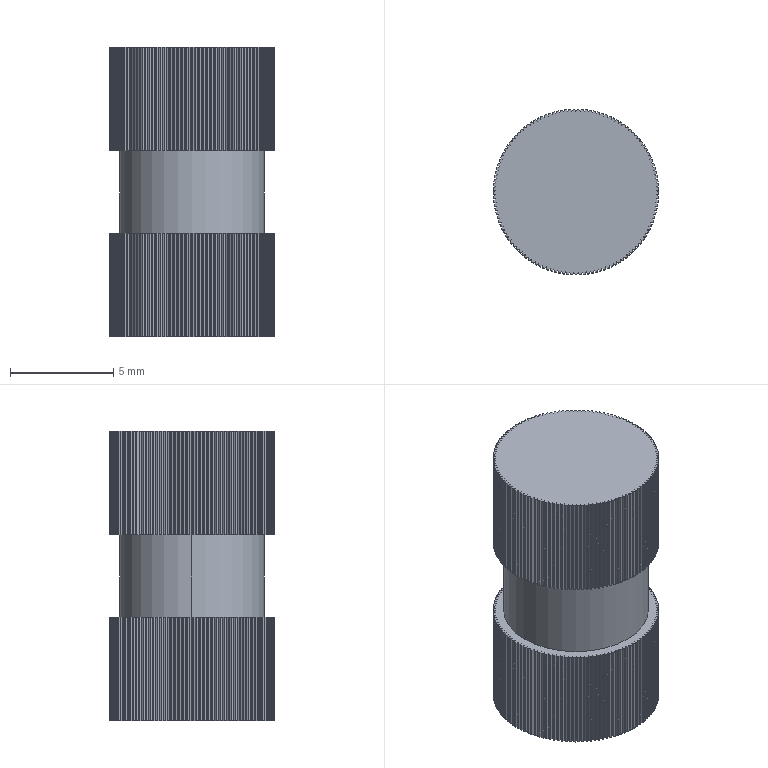Part | NX | features BREP 1 | 1 solid | 761 faces | box 8 x 8 x 14 mm | volume 504.782 mm3 | plane 504 | cylinder 253 | cone 4 | commonest cylinder face diameters 8 x249 4.134 x2 7 x2